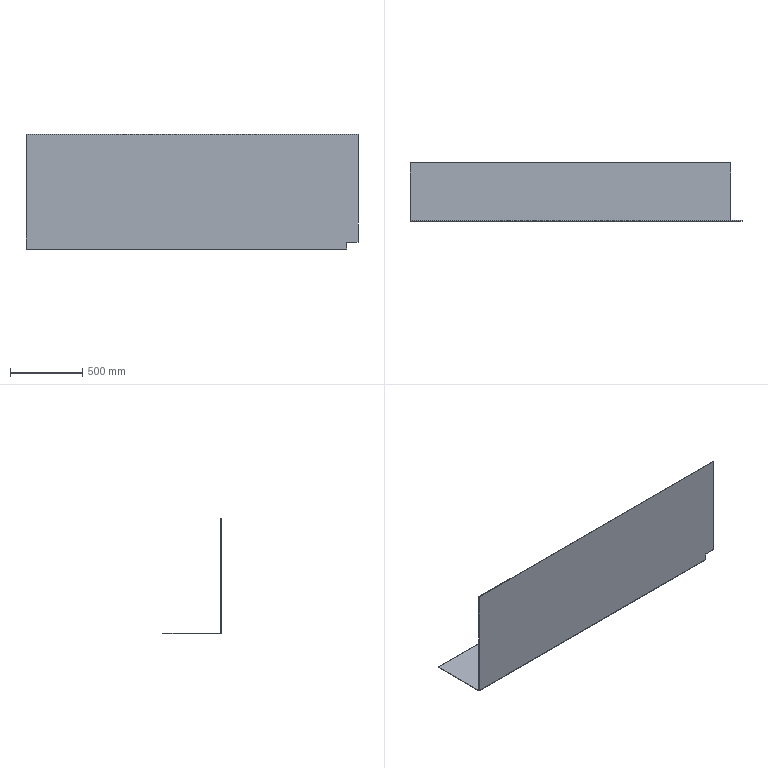Part | STEP file | E3-花纹Plate折弯2 | 1 solid | 14 faces | box 2298 x 403 x 798 mm | volume 8146098 mm3 | plane 12 | cylinder 2 | commonest cylinder face diameters 2 x1 8 x1
STEP:
#1=CARTESIAN_POINT('',(0.,0.,0.));
#2=DIRECTION('',(0.,0.,1.));
#3=DIRECTION('',(1.,0.,0.));
#4=AXIS2_PLACEMENT_3D('',#1,#2,#3);
#5=CARTESIAN_POINT('',(2298.,0.,-746.));
#6=VERTEX_POINT('',#5);
#7=CARTESIAN_POINT('',(2298.,3.,-746.));
#8=VERTEX_POINT('',#7);
#9=CARTESIAN_POINT('',(2298.,3.,-746.));
#10=DIRECTION('',(0.,1.,0.));
#11=VECTOR('',#10,1.);
#12=LINE('',#9,#11);
#13=CARTESIAN_POINT('',(2298.,3.,0.));
#14=DIRECTION('',(1.,0.,0.));
#15=DIRECTION('',(0.,0.,1.));
#16=AXIS2_PLACEMENT_3D('',#13,#14,#15);
#17=PLANE('',#16);
#18=CARTESIAN_POINT('',(-746.,0.));
#19=DIRECTION('',(0.,-1.));
#20=VECTOR('',#19,1.);
#21=LINE('',#18,#20);
#22=(GEOMETRIC_REPRESENTATION_CONTEXT(2)PARAMETRIC_REPRESENTATION_CONTEXT()REPRESENTATION_CONTEXT('',''));
#23=DEFINITIONAL_REPRESENTATION('',(#21),#22);
#24=PCURVE('',#17,#23);
#25=CARTESIAN_POINT('',(2220.,-497.,-746.));
#26=DIRECTION('',(0.,0.,1.));
#27=DIRECTION('',(-1.,0.,0.));
#28=AXIS2_PLACEMENT_3D('',#25,#26,#27);
#29=PLANE('',#28);
#30=CARTESIAN_POINT('',(-78.,-500.));
#31=DIRECTION('',(0.,-1.));
#32=VECTOR('',#31,1.);
#33=LINE('',#30,#32);
#34=(GEOMETRIC_REPRESENTATION_CONTEXT(2)PARAMETRIC_REPRESENTATION_CONTEXT()REPRESENTATION_CONTEXT('',''));
#35=DEFINITIONAL_REPRESENTATION('',(#33),#34);
#36=PCURVE('',#29,#35);
#37=SURFACE_CURVE('',#12,(#24,#36),.PCURVE_S1.);
#38=EDGE_CURVE('',#6,#8,#37,.T.);
#39=ORIENTED_EDGE('',*,*,#38,.T.);
#40=CARTESIAN_POINT('',(2298.,3.,0.));
#41=VERTEX_POINT('',#40);
#42=CARTESIAN_POINT('',(2298.,3.,0.));
#43=DIRECTION('',(0.,0.,1.));
#44=VECTOR('',#43,1.);
#45=LINE('',#42,#44);
#46=CARTESIAN_POINT('',(0.,0.));
#47=DIRECTION('',(1.,0.));
#48=VECTOR('',#47,1.);
#49=LINE('',#46,#48);
#50=(GEOMETRIC_REPRESENTATION_CONTEXT(2)PARAMETRIC_REPRESENTATION_CONTEXT()REPRESENTATION_CONTEXT('',''));
#51=DEFINITIONAL_REPRESENTATION('',(#49),#50);
#52=PCURVE('',#17,#51);
#53=CARTESIAN_POINT('',(0.,3.,0.));
#54=DIRECTION('',(0.,1.,0.));
#55=DIRECTION('',(0.,0.,-1.));
#56=AXIS2_PLACEMENT_3D('',#53,#54,#55);
#57=PLANE('',#56);
#58=CARTESIAN_POINT('',(0.,-2298.));
#59=DIRECTION('',(-1.,0.));
#60=VECTOR('',#59,1.);
#61=LINE('',#58,#60);
#62=(GEOMETRIC_REPRESENTATION_CONTEXT(2)PARAMETRIC_REPRESENTATION_CONTEXT()REPRESENTATION_CONTEXT('',''));
#63=DEFINITIONAL_REPRESENTATION('',(#61),#62);
#64=PCURVE('',#57,#63);
#65=SURFACE_CURVE('',#45,(#52,#64),.PCURVE_S1.);
#66=EDGE_CURVE('',#8,#41,#65,.T.);
#67=ORIENTED_EDGE('',*,*,#66,.T.);
#68=CARTESIAN_POINT('',(2298.,0.,0.));
#69=VERTEX_POINT('',#68);
#70=CARTESIAN_POINT('',(2298.,3.,0.));
#71=DIRECTION('',(0.,1.,0.));
#72=VECTOR('',#71,1.);
#73=LINE('',#70,#72);
#74=CARTESIAN_POINT('',(0.,0.));
#75=DIRECTION('',(0.,-1.));
#76=VECTOR('',#75,1.);
#77=LINE('',#74,#76);
#78=(GEOMETRIC_REPRESENTATION_CONTEXT(2)PARAMETRIC_REPRESENTATION_CONTEXT()REPRESENTATION_CONTEXT('',''));
#79=DEFINITIONAL_REPRESENTATION('',(#77),#78);
#80=PCURVE('',#17,#79);
#81=CARTESIAN_POINT('',(0.,3.,0.));
#82=DIRECTION('',(0.,0.,1.));
#83=DIRECTION('',(-1.,0.,0.));
#84=AXIS2_PLACEMENT_3D('',#81,#82,#83);
#85=PLANE('',#84);
#86=CARTESIAN_POINT('',(-2298.,0.));
#87=DIRECTION('',(0.,-1.));
#88=VECTOR('',#87,1.);
#89=LINE('',#86,#88);
#90=(GEOMETRIC_REPRESENTATION_CONTEXT(2)PARAMETRIC_REPRESENTATION_CONTEXT()REPRESENTATION_CONTEXT('',''));
#91=DEFINITIONAL_REPRESENTATION('',(#89),#90);
#92=PCURVE('',#85,#91);
#93=SURFACE_CURVE('',#73,(#80,#92),.PCURVE_S1.);
#94=EDGE_CURVE('',#69,#41,#93,.T.);
#95=ORIENTED_EDGE('',*,*,#94,.F.);
#96=CARTESIAN_POINT('',(2298.,0.,0.));
#97=DIRECTION('',(0.,0.,1.));
#98=VECTOR('',#97,1.);
#99=LINE('',#96,#98);
#100=CARTESIAN_POINT('',(0.,3.));
#101=DIRECTION('',(1.,0.));
#102=VECTOR('',#101,1.);
#103=LINE('',#100,#102);
#104=(GEOMETRIC_REPRESENTATION_CONTEXT(2)PARAMETRIC_REPRESENTATION_CONTEXT()REPRESENTATION_CONTEXT('',''));
#105=DEFINITIONAL_REPRESENTATION('',(#103),#104);
#106=PCURVE('',#17,#105);
#107=CARTESIAN_POINT('',(0.,0.,0.));
#108=DIRECTION('',(0.,1.,0.));
#109=DIRECTION('',(0.,0.,-1.));
#110=AXIS2_PLACEMENT_3D('',#107,#108,#109);
#111=PLANE('',#110);
#112=CARTESIAN_POINT('',(0.,-2298.));
#113=DIRECTION('',(-1.,0.));
#114=VECTOR('',#113,1.);
#115=LINE('',#112,#114);
#116=(GEOMETRIC_REPRESENTATION_CONTEXT(2)PARAMETRIC_REPRESENTATION_CONTEXT()REPRESENTATION_CONTEXT('',''));
#117=DEFINITIONAL_REPRESENTATION('',(#115),#116);
#118=PCURVE('',#111,#117);
#119=SURFACE_CURVE('',#99,(#106,#118),.PCURVE_S1.);
#120=EDGE_CURVE('',#6,#69,#119,.T.);
#121=ORIENTED_EDGE('',*,*,#120,.F.);
#122=EDGE_LOOP('',(#39,#67,#95,#121));
#123=FACE_BOUND('',#122,.T.);
#124=ADVANCED_FACE('',(#123),#17,.T.);
#125=CARTESIAN_POINT('',(2220.,3.,-746.));
#126=VERTEX_POINT('',#125);
#127=CARTESIAN_POINT('',(2220.,3.,-794.));
#128=VERTEX_POINT('',#127);
#129=CARTESIAN_POINT('',(2220.,3.,0.));
#130=DIRECTION('',(0.,0.,-1.));
#131=VECTOR('',#130,1.);
#132=LINE('',#129,#131);
#133=CARTESIAN_POINT('',(0.,-2220.));
#134=DIRECTION('',(1.,0.));
#135=VECTOR('',#134,1.);
#136=LINE('',#133,#135);
#137=(GEOMETRIC_REPRESENTATION_CONTEXT(2)PARAMETRIC_REPRESENTATION_CONTEXT()REPRESENTATION_CONTEXT('',''));
#138=DEFINITIONAL_REPRESENTATION('',(#136),#137);
#139=PCURVE('',#57,#138);
#140=CARTESIAN_POINT('',(2220.,-497.,-798.));
#141=DIRECTION('',(-1.,0.,0.));
#142=DIRECTION('',(0.,0.,-1.));
#143=AXIS2_PLACEMENT_3D('',#140,#141,#142);
#144=PLANE('',#143);
#145=CARTESIAN_POINT('',(-798.,-500.));
#146=DIRECTION('',(1.,0.));
#147=VECTOR('',#146,1.);
#148=LINE('',#145,#147);
#149=(GEOMETRIC_REPRESENTATION_CONTEXT(2)PARAMETRIC_REPRESENTATION_CONTEXT()REPRESENTATION_CONTEXT('',''));
#150=DEFINITIONAL_REPRESENTATION('',(#148),#149);
#151=PCURVE('',#144,#150);
#152=SURFACE_CURVE('',#132,(#139,#151),.PCURVE_S1.);
#153=EDGE_CURVE('',#126,#128,#152,.T.);
#154=ORIENTED_EDGE('',*,*,#153,.T.);
#155=CARTESIAN_POINT('',(0.,3.,-794.));
#156=VERTEX_POINT('',#155);
#157=CARTESIAN_POINT('',(2298.,3.,-794.));
#158=DIRECTION('',(-1.,0.,0.));
#159=VECTOR('',#158,1.);
#160=LINE('',#157,#159);
#161=CARTESIAN_POINT('',(794.,-2298.));
#162=DIRECTION('',(0.,1.));
#163=VECTOR('',#162,1.);
#164=LINE('',#161,#163);
#165=(GEOMETRIC_REPRESENTATION_CONTEXT(2)PARAMETRIC_REPRESENTATION_CONTEXT()REPRESENTATION_CONTEXT('',''));
#166=DEFINITIONAL_REPRESENTATION('',(#164),#165);
#167=PCURVE('',#57,#166);
#168=CARTESIAN_POINT('',(2298.,4.,-794.));
#169=DIRECTION('',(1.,0.,0.));
#170=DIRECTION('',(0.,0.,-1.));
#171=AXIS2_PLACEMENT_3D('',#168,#169,#170);
#172=CYLINDRICAL_SURFACE('',#171,1.);
#173=CARTESIAN_POINT('',(4.712,0.));
#174=DIRECTION('',(0.,-1.));
#175=VECTOR('',#174,1.);
#176=LINE('',#173,#175);
#177=(GEOMETRIC_REPRESENTATION_CONTEXT(2)PARAMETRIC_REPRESENTATION_CONTEXT()REPRESENTATION_CONTEXT('',''));
#178=DEFINITIONAL_REPRESENTATION('',(#176),#177);
#179=PCURVE('',#172,#178);
#180=SURFACE_CURVE('',#160,(#167,#179),.PCURVE_S1.);
#181=EDGE_CURVE('',#128,#156,#180,.T.);
#182=ORIENTED_EDGE('',*,*,#181,.T.);
#183=CARTESIAN_POINT('',(0.,3.,0.));
#184=VERTEX_POINT('',#183);
#185=CARTESIAN_POINT('',(0.,3.,0.));
#186=DIRECTION('',(0.,0.,-1.));
#187=VECTOR('',#186,1.);
#188=LINE('',#185,#187);
#189=CARTESIAN_POINT('',(0.,0.));
#190=DIRECTION('',(1.,0.));
#191=VECTOR('',#190,1.);
#192=LINE('',#189,#191);
#193=(GEOMETRIC_REPRESENTATION_CONTEXT(2)PARAMETRIC_REPRESENTATION_CONTEXT()REPRESENTATION_CONTEXT('',''));
#194=DEFINITIONAL_REPRESENTATION('',(#192),#193);
#195=PCURVE('',#57,#194);
#196=CARTESIAN_POINT('',(0.,3.,0.));
#197=DIRECTION('',(-1.,0.,0.));
#198=DIRECTION('',(0.,0.,-1.));
#199=AXIS2_PLACEMENT_3D('',#196,#197,#198);
#200=PLANE('',#199);
#201=CARTESIAN_POINT('',(0.,0.));
#202=DIRECTION('',(1.,0.));
#203=VECTOR('',#202,1.);
#204=LINE('',#201,#203);
#205=(GEOMETRIC_REPRESENTATION_CONTEXT(2)PARAMETRIC_REPRESENTATION_CONTEXT()REPRESENTATION_CONTEXT('',''));
#206=DEFINITIONAL_REPRESENTATION('',(#204),#205);
#207=PCURVE('',#200,#206);
#208=SURFACE_CURVE('',#188,(#195,#207),.PCURVE_S1.);
#209=EDGE_CURVE('',#184,#156,#208,.T.);
#210=ORIENTED_EDGE('',*,*,#209,.F.);
#211=CARTESIAN_POINT('',(0.,3.,0.));
#212=DIRECTION('',(-1.,0.,0.));
#213=VECTOR('',#212,1.);
#214=LINE('',#211,#213);
#215=CARTESIAN_POINT('',(0.,0.));
#216=DIRECTION('',(0.,1.));
#217=VECTOR('',#216,1.);
#218=LINE('',#215,#217);
#219=(GEOMETRIC_REPRESENTATION_CONTEXT(2)PARAMETRIC_REPRESENTATION_CONTEXT()REPRESENTATION_CONTEXT('',''));
#220=DEFINITIONAL_REPRESENTATION('',(#218),#219);
#221=PCURVE('',#57,#220);
#222=CARTESIAN_POINT('',(0.,0.));
#223=DIRECTION('',(1.,0.));
#224=VECTOR('',#223,1.);
#225=LINE('',#222,#224);
#226=(GEOMETRIC_REPRESENTATION_CONTEXT(2)PARAMETRIC_REPRESENTATION_CONTEXT()REPRESENTATION_CONTEXT('',''));
#227=DEFINITIONAL_REPRESENTATION('',(#225),#226);
#228=PCURVE('',#85,#227);
#229=SURFACE_CURVE('',#214,(#221,#228),.PCURVE_S1.);
#230=EDGE_CURVE('',#41,#184,#229,.T.);
#231=ORIENTED_EDGE('',*,*,#230,.F.);
#232=ORIENTED_EDGE('',*,*,#66,.F.);
#233=CARTESIAN_POINT('',(0.,3.,-746.));
#234=DIRECTION('',(-1.,0.,0.));
#235=VECTOR('',#234,1.);
#236=LINE('',#233,#235);
#237=CARTESIAN_POINT('',(746.,0.));
#238=DIRECTION('',(0.,1.));
#239=VECTOR('',#238,1.);
#240=LINE('',#237,#239);
#241=(GEOMETRIC_REPRESENTATION_CONTEXT(2)PARAMETRIC_REPRESENTATION_CONTEXT()REPRESENTATION_CONTEXT('',''));
#242=DEFINITIONAL_REPRESENTATION('',(#240),#241);
#243=PCURVE('',#57,#242);
#244=CARTESIAN_POINT('',(2220.,-500.));
#245=DIRECTION('',(1.,0.));
#246=VECTOR('',#245,1.);
#247=LINE('',#244,#246);
#248=(GEOMETRIC_REPRESENTATION_CONTEXT(2)PARAMETRIC_REPRESENTATION_CONTEXT()REPRESENTATION_CONTEXT('',''));
#249=DEFINITIONAL_REPRESENTATION('',(#247),#248);
#250=PCURVE('',#29,#249);
#251=SURFACE_CURVE('',#236,(#243,#250),.PCURVE_S1.);
#252=EDGE_CURVE('',#8,#126,#251,.T.);
#253=ORIENTED_EDGE('',*,*,#252,.T.);
#254=EDGE_LOOP('',(#154,#182,#210,#231,#232,#253));
#255=FACE_BOUND('',#254,.T.);
#256=ADVANCED_FACE('',(#255),#57,.T.);
#257=CARTESIAN_POINT('',(2220.,0.,-746.));
#258=VERTEX_POINT('',#257);
#259=CARTESIAN_POINT('',(0.,0.,-746.));
#260=DIRECTION('',(-1.,0.,0.));
#261=VECTOR('',#260,1.);
#262=LINE('',#259,#261);
#263=CARTESIAN_POINT('',(746.,0.));
#264=DIRECTION('',(0.,1.));
#265=VECTOR('',#264,1.);
#266=LINE('',#263,#265);
#267=(GEOMETRIC_REPRESENTATION_CONTEXT(2)PARAMETRIC_REPRESENTATION_CONTEXT()REPRESENTATION_CONTEXT('',''));
#268=DEFINITIONAL_REPRESENTATION('',(#266),#267);
#269=PCURVE('',#111,#268);
#270=CARTESIAN_POINT('',(2220.,-497.));
#271=DIRECTION('',(1.,0.));
#272=VECTOR('',#271,1.);
#273=LINE('',#270,#272);
#274=(GEOMETRIC_REPRESENTATION_CONTEXT(2)PARAMETRIC_REPRESENTATION_CONTEXT()REPRESENTATION_CONTEXT('',''));
#275=DEFINITIONAL_REPRESENTATION('',(#273),#274);
#276=PCURVE('',#29,#275);
#277=SURFACE_CURVE('',#262,(#269,#276),.PCURVE_S1.);
#278=EDGE_CURVE('',#6,#258,#277,.T.);
#279=ORIENTED_EDGE('',*,*,#278,.F.);
#280=ORIENTED_EDGE('',*,*,#120,.T.);
#281=CARTESIAN_POINT('',(0.,0.,0.));
#282=VERTEX_POINT('',#281);
#283=CARTESIAN_POINT('',(0.,0.,0.));
#284=DIRECTION('',(-1.,0.,0.));
#285=VECTOR('',#284,1.);
#286=LINE('',#283,#285);
#287=CARTESIAN_POINT('',(0.,0.));
#288=DIRECTION('',(0.,1.));
#289=VECTOR('',#288,1.);
#290=LINE('',#287,#289);
#291=(GEOMETRIC_REPRESENTATION_CONTEXT(2)PARAMETRIC_REPRESENTATION_CONTEXT()REPRESENTATION_CONTEXT('',''));
#292=DEFINITIONAL_REPRESENTATION('',(#290),#291);
#293=PCURVE('',#111,#292);
#294=CARTESIAN_POINT('',(0.,3.));
#295=DIRECTION('',(1.,0.));
#296=VECTOR('',#295,1.);
#297=LINE('',#294,#296);
#298=(GEOMETRIC_REPRESENTATION_CONTEXT(2)PARAMETRIC_REPRESENTATION_CONTEXT()REPRESENTATION_CONTEXT('',''));
#299=DEFINITIONAL_REPRESENTATION('',(#297),#298);
#300=PCURVE('',#85,#299);
#301=SURFACE_CURVE('',#286,(#293,#300),.PCURVE_S1.);
#302=EDGE_CURVE('',#69,#282,#301,.T.);
#303=ORIENTED_EDGE('',*,*,#302,.T.);
#304=CARTESIAN_POINT('',(0.,0.,-794.));
#305=VERTEX_POINT('',#304);
#306=CARTESIAN_POINT('',(0.,0.,0.));
#307=DIRECTION('',(0.,0.,-1.));
#308=VECTOR('',#307,1.);
#309=LINE('',#306,#308);
#310=CARTESIAN_POINT('',(0.,0.));
#311=DIRECTION('',(1.,0.));
#312=VECTOR('',#311,1.);
#313=LINE('',#310,#312);
#314=(GEOMETRIC_REPRESENTATION_CONTEXT(2)PARAMETRIC_REPRESENTATION_CONTEXT()REPRESENTATION_CONTEXT('',''));
#315=DEFINITIONAL_REPRESENTATION('',(#313),#314);
#316=PCURVE('',#111,#315);
#317=CARTESIAN_POINT('',(0.,3.));
#318=DIRECTION('',(1.,0.));
#319=VECTOR('',#318,1.);
#320=LINE('',#317,#319);
#321=(GEOMETRIC_REPRESENTATION_CONTEXT(2)PARAMETRIC_REPRESENTATION_CONTEXT()REPRESENTATION_CONTEXT('',''));
#322=DEFINITIONAL_REPRESENTATION('',(#320),#321);
#323=PCURVE('',#200,#322);
#324=SURFACE_CURVE('',#309,(#316,#323),.PCURVE_S1.);
#325=EDGE_CURVE('',#282,#305,#324,.T.);
#326=ORIENTED_EDGE('',*,*,#325,.T.);
#327=CARTESIAN_POINT('',(2220.,0.,-794.));
#328=VERTEX_POINT('',#327);
#329=CARTESIAN_POINT('',(2298.,0.,-794.));
#330=DIRECTION('',(-1.,0.,0.));
#331=VECTOR('',#330,1.);
#332=LINE('',#329,#331);
#333=CARTESIAN_POINT('',(794.,-2298.));
#334=DIRECTION('',(0.,1.));
#335=VECTOR('',#334,1.);
#336=LINE('',#333,#335);
#337=(GEOMETRIC_REPRESENTATION_CONTEXT(2)PARAMETRIC_REPRESENTATION_CONTEXT()REPRESENTATION_CONTEXT('',''));
#338=DEFINITIONAL_REPRESENTATION('',(#336),#337);
#339=PCURVE('',#111,#338);
#340=CARTESIAN_POINT('',(2298.,4.,-794.));
#341=DIRECTION('',(1.,0.,0.));
#342=DIRECTION('',(0.,0.,-1.));
#343=AXIS2_PLACEMENT_3D('',#340,#341,#342);
#344=CYLINDRICAL_SURFACE('',#343,4.);
#345=CARTESIAN_POINT('',(4.712,0.));
#346=DIRECTION('',(0.,-1.));
#347=VECTOR('',#346,1.);
#348=LINE('',#345,#347);
#349=(GEOMETRIC_REPRESENTATION_CONTEXT(2)PARAMETRIC_REPRESENTATION_CONTEXT()REPRESENTATION_CONTEXT('',''));
#350=DEFINITIONAL_REPRESENTATION('',(#348),#349);
#351=PCURVE('',#344,#350);
#352=SURFACE_CURVE('',#332,(#339,#351),.PCURVE_S1.);
#353=EDGE_CURVE('',#328,#305,#352,.T.);
#354=ORIENTED_EDGE('',*,*,#353,.F.);
#355=CARTESIAN_POINT('',(2220.,0.,0.));
#356=DIRECTION('',(0.,0.,-1.));
#357=VECTOR('',#356,1.);
#358=LINE('',#355,#357);
#359=CARTESIAN_POINT('',(0.,-2220.));
#360=DIRECTION('',(1.,0.));
#361=VECTOR('',#360,1.);
#362=LINE('',#359,#361);
#363=(GEOMETRIC_REPRESENTATION_CONTEXT(2)PARAMETRIC_REPRESENTATION_CONTEXT()REPRESENTATION_CONTEXT('',''));
#364=DEFINITIONAL_REPRESENTATION('',(#362),#363);
#365=PCURVE('',#111,#364);
#366=CARTESIAN_POINT('',(-798.,-497.));
#367=DIRECTION('',(1.,0.));
#368=VECTOR('',#367,1.);
#369=LINE('',#366,#368);
#370=(GEOMETRIC_REPRESENTATION_CONTEXT(2)PARAMETRIC_REPRESENTATION_CONTEXT()REPRESENTATION_CONTEXT('',''));
#371=DEFINITIONAL_REPRESENTATION('',(#369),#370);
#372=PCURVE('',#144,#371);
#373=SURFACE_CURVE('',#358,(#365,#372),.PCURVE_S1.);
#374=EDGE_CURVE('',#258,#328,#373,.T.);
#375=ORIENTED_EDGE('',*,*,#374,.F.);
#376=EDGE_LOOP('',(#279,#280,#303,#326,#354,#375));
#377=FACE_BOUND('',#376,.T.);
#378=ADVANCED_FACE('',(#377),#111,.F.);
#379=ORIENTED_EDGE('',*,*,#94,.T.);
#380=ORIENTED_EDGE('',*,*,#230,.T.);
#381=CARTESIAN_POINT('',(0.,3.,0.));
#382=DIRECTION('',(0.,1.,0.));
#383=VECTOR('',#382,1.);
#384=LINE('',#381,#383);
#385=CARTESIAN_POINT('',(0.,0.));
#386=DIRECTION('',(0.,-1.));
#387=VECTOR('',#386,1.);
#388=LINE('',#385,#387);
#389=(GEOMETRIC_REPRESENTATION_CONTEXT(2)PARAMETRIC_REPRESENTATION_CONTEXT()REPRESENTATION_CONTEXT('',''));
#390=DEFINITIONAL_REPRESENTATION('',(#388),#389);
#391=PCURVE('',#85,#390);
#392=CARTESIAN_POINT('',(0.,0.));
#393=DIRECTION('',(0.,-1.));
#394=VECTOR('',#393,1.);
#395=LINE('',#392,#394);
#396=(GEOMETRIC_REPRESENTATION_CONTEXT(2)PARAMETRIC_REPRESENTATION_CONTEXT()REPRESENTATION_CONTEXT('',''));
#397=DEFINITIONAL_REPRESENTATION('',(#395),#396);
#398=PCURVE('',#200,#397);
#399=SURFACE_CURVE('',#384,(#391,#398),.PCURVE_S1.);
#400=EDGE_CURVE('',#282,#184,#399,.T.);
#401=ORIENTED_EDGE('',*,*,#400,.F.);
#402=ORIENTED_EDGE('',*,*,#302,.F.);
#403=EDGE_LOOP('',(#379,#380,#401,#402));
#404=FACE_BOUND('',#403,.T.);
#405=ADVANCED_FACE('',(#404),#85,.T.);
#406=CARTESIAN_POINT('',(0.,3.,-794.));
#407=DIRECTION('',(0.,-1.,0.));
#408=VECTOR('',#407,1.);
#409=LINE('',#406,#408);
#410=CARTESIAN_POINT('',(794.,0.));
#411=DIRECTION('',(0.,1.));
#412=VECTOR('',#411,1.);
#413=LINE('',#410,#412);
#414=(GEOMETRIC_REPRESENTATION_CONTEXT(2)PARAMETRIC_REPRESENTATION_CONTEXT()REPRESENTATION_CONTEXT('',''));
#415=DEFINITIONAL_REPRESENTATION('',(#413),#414);
#416=PCURVE('',#200,#415);
#417=CARTESIAN_POINT('',(0.,4.,-794.));
#418=DIRECTION('',(-1.,0.,0.));
#419=DIRECTION('',(0.,0.,-1.));
#420=AXIS2_PLACEMENT_3D('',#417,#418,#419);
#421=PLANE('',#420);
#422=CARTESIAN_POINT('',(0.,1.));
#423=DIRECTION('',(0.,1.));
#424=VECTOR('',#423,1.);
#425=LINE('',#422,#424);
#426=(GEOMETRIC_REPRESENTATION_CONTEXT(2)PARAMETRIC_REPRESENTATION_CONTEXT()REPRESENTATION_CONTEXT('',''));
#427=DEFINITIONAL_REPRESENTATION('',(#425),#426);
#428=PCURVE('',#421,#427);
#429=SURFACE_CURVE('',#409,(#416,#428),.PCURVE_S1.);
#430=EDGE_CURVE('',#156,#305,#429,.T.);
#431=ORIENTED_EDGE('',*,*,#430,.T.);
#432=ORIENTED_EDGE('',*,*,#325,.F.);
#433=ORIENTED_EDGE('',*,*,#400,.T.);
#434=ORIENTED_EDGE('',*,*,#209,.T.);
#435=EDGE_LOOP('',(#431,#432,#433,#434));
#436=FACE_BOUND('',#435,.T.);
#437=ADVANCED_FACE('',(#436),#200,.T.);
#438=CARTESIAN_POINT('',(0.,4.,-795.));
#439=VERTEX_POINT('',#438);
#440=CARTESIAN_POINT('',(0.,4.,-798.));
#441=VERTEX_POINT('',#440);
#442=CARTESIAN_POINT('',(0.,4.,-798.));
#443=DIRECTION('',(0.,0.,-1.));
#444=VECTOR('',#443,1.);
#445=LINE('',#442,#444);
#446=CARTESIAN_POINT('',(4.,0.));
#447=DIRECTION('',(1.,0.));
#448=VECTOR('',#447,1.);
#449=LINE('',#446,#448);
#450=(GEOMETRIC_REPRESENTATION_CONTEXT(2)PARAMETRIC_REPRESENTATION_CONTEXT()REPRESENTATION_CONTEXT('',''));
#451=DEFINITIONAL_REPRESENTATION('',(#449),#450);
#452=PCURVE('',#421,#451);
#453=CARTESIAN_POINT('',(0.,3.,-798.));
#454=DIRECTION('',(1.,0.,0.));
#455=DIRECTION('',(0.,0.,1.));
#456=AXIS2_PLACEMENT_3D('',#453,#454,#455);
#457=PLANE('',#456);
#458=CARTESIAN_POINT('',(0.,-1.));
#459=DIRECTION('',(-1.,0.));
#460=VECTOR('',#459,1.);
#461=LINE('',#458,#460);
#462=(GEOMETRIC_REPRESENTATION_CONTEXT(2)PARAMETRIC_REPRESENTATION_CONTEXT()REPRESENTATION_CONTEXT('',''));
#463=DEFINITIONAL_REPRESENTATION('',(#461),#462);
#464=PCURVE('',#457,#463);
#465=SURFACE_CURVE('',#445,(#452,#464),.PCURVE_S1.);
#466=EDGE_CURVE('',#439,#441,#465,.T.);
#467=ORIENTED_EDGE('',*,*,#466,.T.);
#468=CARTESIAN_POINT('',(0.,4.,-794.));
#469=DIRECTION('',(1.,0.,0.));
#470=DIRECTION('',(0.,0.,1.));
#471=AXIS2_PLACEMENT_3D('',#468,#469,#470);
#472=CIRCLE('',#471,4.);
#473=CARTESIAN_POINT('',(-4.,0.));
#474=CARTESIAN_POINT('',(-4.,6.928));
#475=CARTESIAN_POINT('',(2.,3.464));
#476=CARTESIAN_POINT('',(8.,0.));
#477=CARTESIAN_POINT('',(2.,-3.464));
#478=CARTESIAN_POINT('',(-4.,-6.928));
#479=CARTESIAN_POINT('',(-4.,0.));
#480=(BOUNDED_CURVE()B_SPLINE_CURVE(2,(#473,#474,#475,#476,#477,#478,#479),.UNSPECIFIED.,.T.,.F.)B_SPLINE_CURVE_WITH_KNOTS((1,2,2,2,2,1),(-2.094,0.,2.094,4.189,6.283,8.378),.UNSPECIFIED.)CURVE()GEOMETRIC_REPRESENTATION_ITEM()RATIONAL_B_SPLINE_CURVE((1.,0.5,1.,0.5,1.,0.5,1.))REPRESENTATION_ITEM(''));
#481=(GEOMETRIC_REPRESENTATION_CONTEXT(2)PARAMETRIC_REPRESENTATION_CONTEXT()REPRESENTATION_CONTEXT('',''));
#482=DEFINITIONAL_REPRESENTATION('',(#480),#481);
#483=PCURVE('',#421,#482);
#484=CARTESIAN_POINT('',(3.142,-2298.));
#485=DIRECTION('',(1.,0.));
#486=VECTOR('',#485,1.);
#487=LINE('',#484,#486);
#488=(GEOMETRIC_REPRESENTATION_CONTEXT(2)PARAMETRIC_REPRESENTATION_CONTEXT()REPRESENTATION_CONTEXT('',''));
#489=DEFINITIONAL_REPRESENTATION('',(#487),#488);
#490=PCURVE('',#344,#489);
#491=SURFACE_CURVE('',#472,(#483,#490),.PCURVE_S1.);
#492=EDGE_CURVE('',#305,#441,#491,.T.);
#493=ORIENTED_EDGE('',*,*,#492,.F.);
#494=ORIENTED_EDGE('',*,*,#430,.F.);
#495=CARTESIAN_POINT('',(0.,4.,-794.));
#496=DIRECTION('',(1.,0.,0.));
#497=DIRECTION('',(0.,0.,1.));
#498=AXIS2_PLACEMENT_3D('',#495,#496,#497);
#499=CIRCLE('',#498,1.);
#500=CARTESIAN_POINT('',(-1.,0.));
#501=CARTESIAN_POINT('',(-1.,1.732));
#502=CARTESIAN_POINT('',(0.5,0.866));
#503=CARTESIAN_POINT('',(2.,0.));
#504=CARTESIAN_POINT('',(0.5,-0.866));
#505=CARTESIAN_POINT('',(-1.,-1.732));
#506=CARTESIAN_POINT('',(-1.,0.));
#507=(BOUNDED_CURVE()B_SPLINE_CURVE(2,(#500,#501,#502,#503,#504,#505,#506),.UNSPECIFIED.,.T.,.F.)B_SPLINE_CURVE_WITH_KNOTS((1,2,2,2,2,1),(-2.094,0.,2.094,4.189,6.283,8.378),.UNSPECIFIED.)CURVE()GEOMETRIC_REPRESENTATION_ITEM()RATIONAL_B_SPLINE_CURVE((1.,0.5,1.,0.5,1.,0.5,1.))REPRESENTATION_ITEM(''));
#508=(GEOMETRIC_REPRESENTATION_CONTEXT(2)PARAMETRIC_REPRESENTATION_CONTEXT()REPRESENTATION_CONTEXT('',''));
#509=DEFINITIONAL_REPRESENTATION('',(#507),#508);
#510=PCURVE('',#421,#509);
#511=CARTESIAN_POINT('',(3.142,-2298.));
#512=DIRECTION('',(1.,0.));
#513=VECTOR('',#512,1.);
#514=LINE('',#511,#513);
#515=(GEOMETRIC_REPRESENTATION_CONTEXT(2)PARAMETRIC_REPRESENTATION_CONTEXT()REPRESENTATION_CONTEXT('',''));
#516=DEFINITIONAL_REPRESENTATION('',(#514),#515);
#517=PCURVE('',#172,#516);
#518=SURFACE_CURVE('',#499,(#510,#517),.PCURVE_S1.);
#519=EDGE_CURVE('',#156,#439,#518,.T.);
#520=ORIENTED_EDGE('',*,*,#519,.T.);
#521=EDGE_LOOP('',(#467,#493,#494,#520));
#522=FACE_BOUND('',#521,.T.);
#523=ADVANCED_FACE('',(#522),#421,.T.);
#524=CARTESIAN_POINT('',(2220.,4.,-798.));
#525=VERTEX_POINT('',#524);
#526=CARTESIAN_POINT('',(2220.,4.,-794.));
#527=DIRECTION('',(-1.,0.,0.));
#528=DIRECTION('',(0.,0.,-1.));
#529=AXIS2_PLACEMENT_3D('',#526,#527,#528);
#530=CIRCLE('',#529,4.);
#531=CARTESIAN_POINT('',(6.283,-78.));
#532=DIRECTION('',(-1.,0.));
#533=VECTOR('',#532,1.);
#534=LINE('',#531,#533);
#535=(GEOMETRIC_REPRESENTATION_CONTEXT(2)PARAMETRIC_REPRESENTATION_CONTEXT()REPRESENTATION_CONTEXT('',''));
#536=DEFINITIONAL_REPRESENTATION('',(#534),#535);
#537=PCURVE('',#344,#536);
#538=CARTESIAN_POINT('',(-4.,-501.));
#539=DIRECTION('',(1.,0.));
#540=AXIS2_PLACEMENT_2D('',#538,#539);
#541=CIRCLE('',#540,4.);
#542=(GEOMETRIC_REPRESENTATION_CONTEXT(2)PARAMETRIC_REPRESENTATION_CONTEXT()REPRESENTATION_CONTEXT('',''));
#543=DEFINITIONAL_REPRESENTATION('',(#541),#542);
#544=PCURVE('',#144,#543);
#545=SURFACE_CURVE('',#530,(#537,#544),.PCURVE_S1.);
#546=EDGE_CURVE('',#525,#328,#545,.T.);
#547=ORIENTED_EDGE('',*,*,#546,.T.);
#548=ORIENTED_EDGE('',*,*,#353,.T.);
#549=ORIENTED_EDGE('',*,*,#492,.T.);
#550=CARTESIAN_POINT('',(0.,4.,-798.));
#551=DIRECTION('',(-1.,0.,0.));
#552=VECTOR('',#551,1.);
#553=LINE('',#550,#552);
#554=CARTESIAN_POINT('',(6.283,-2298.));
#555=DIRECTION('',(0.,-1.));
#556=VECTOR('',#555,1.);
#557=LINE('',#554,#556);
#558=(GEOMETRIC_REPRESENTATION_CONTEXT(2)PARAMETRIC_REPRESENTATION_CONTEXT()REPRESENTATION_CONTEXT('',''));
#559=DEFINITIONAL_REPRESENTATION('',(#557),#558);
#560=PCURVE('',#344,#559);
#561=CARTESIAN_POINT('',(0.,0.,-798.));
#562=DIRECTION('',(0.,0.,1.));
#563=DIRECTION('',(-1.,0.,0.));
#564=AXIS2_PLACEMENT_3D('',#561,#562,#563);
#565=PLANE('',#564);
#566=CARTESIAN_POINT('',(0.,-4.));
#567=DIRECTION('',(1.,0.));
#568=VECTOR('',#567,1.);
#569=LINE('',#566,#568);
#570=(GEOMETRIC_REPRESENTATION_CONTEXT(2)PARAMETRIC_REPRESENTATION_CONTEXT()REPRESENTATION_CONTEXT('',''));
#571=DEFINITIONAL_REPRESENTATION('',(#569),#570);
#572=PCURVE('',#565,#571);
#573=SURFACE_CURVE('',#553,(#560,#572),.PCURVE_S1.);
#574=EDGE_CURVE('',#525,#441,#573,.T.);
#575=ORIENTED_EDGE('',*,*,#574,.F.);
#576=EDGE_LOOP('',(#547,#548,#549,#575));
#577=FACE_BOUND('',#576,.T.);
#578=ADVANCED_FACE('',(#577),#344,.T.);
#579=CARTESIAN_POINT('',(2220.,4.,-795.));
#580=VERTEX_POINT('',#579);
#581=CARTESIAN_POINT('',(2220.,4.,-794.));
#582=DIRECTION('',(-1.,0.,0.));
#583=DIRECTION('',(0.,0.,-1.));
#584=AXIS2_PLACEMENT_3D('',#581,#582,#583);
#585=CIRCLE('',#584,1.);
#586=CARTESIAN_POINT('',(6.283,-78.));
#587=DIRECTION('',(-1.,0.));
#588=VECTOR('',#587,1.);
#589=LINE('',#586,#588);
#590=(GEOMETRIC_REPRESENTATION_CONTEXT(2)PARAMETRIC_REPRESENTATION_CONTEXT()REPRESENTATION_CONTEXT('',''));
#591=DEFINITIONAL_REPRESENTATION('',(#589),#590);
#592=PCURVE('',#172,#591);
#593=CARTESIAN_POINT('',(-4.,-501.));
#594=DIRECTION('',(1.,0.));
#595=AXIS2_PLACEMENT_2D('',#593,#594);
#596=CIRCLE('',#595,1.);
#597=(GEOMETRIC_REPRESENTATION_CONTEXT(2)PARAMETRIC_REPRESENTATION_CONTEXT()REPRESENTATION_CONTEXT('',''));
#598=DEFINITIONAL_REPRESENTATION('',(#596),#597);
#599=PCURVE('',#144,#598);
#600=SURFACE_CURVE('',#585,(#592,#599),.PCURVE_S1.);
#601=EDGE_CURVE('',#580,#128,#600,.T.);
#602=ORIENTED_EDGE('',*,*,#601,.T.);
#603=ORIENTED_EDGE('',*,*,#181,.T.);
#604=ORIENTED_EDGE('',*,*,#519,.T.);
#605=CARTESIAN_POINT('',(0.,4.,-795.));
#606=DIRECTION('',(1.,0.,0.));
#607=VECTOR('',#606,1.);
#608=LINE('',#605,#607);
#609=CARTESIAN_POINT('',(6.283,-2298.));
#610=DIRECTION('',(0.,1.));
#611=VECTOR('',#610,1.);
#612=LINE('',#609,#611);
#613=(GEOMETRIC_REPRESENTATION_CONTEXT(2)PARAMETRIC_REPRESENTATION_CONTEXT()REPRESENTATION_CONTEXT('',''));
#614=DEFINITIONAL_REPRESENTATION('',(#612),#613);
#615=PCURVE('',#172,#614);
#616=CARTESIAN_POINT('',(0.,0.,-795.));
#617=DIRECTION('',(0.,0.,1.));
#618=DIRECTION('',(-1.,0.,0.));
#619=AXIS2_PLACEMENT_3D('',#616,#617,#618);
#620=PLANE('',#619);
#621=CARTESIAN_POINT('',(0.,-4.));
#622=DIRECTION('',(-1.,0.));
#623=VECTOR('',#622,1.);
#624=LINE('',#621,#623);
#625=(GEOMETRIC_REPRESENTATION_CONTEXT(2)PARAMETRIC_REPRESENTATION_CONTEXT()REPRESENTATION_CONTEXT('',''));
#626=DEFINITIONAL_REPRESENTATION('',(#624),#625);
#627=PCURVE('',#620,#626);
#628=SURFACE_CURVE('',#608,(#615,#627),.PCURVE_S1.);
#629=EDGE_CURVE('',#439,#580,#628,.T.);
#630=ORIENTED_EDGE('',*,*,#629,.T.);
#631=EDGE_LOOP('',(#602,#603,#604,#630));
#632=FACE_BOUND('',#631,.F.);
#633=ADVANCED_FACE('',(#632),#172,.F.);
#634=ORIENTED_EDGE('',*,*,#466,.F.);
#635=CARTESIAN_POINT('',(0.,403.,-795.));
#636=VERTEX_POINT('',#635);
#637=CARTESIAN_POINT('',(0.,3.,-795.));
#638=DIRECTION('',(0.,-1.,0.));
#639=VECTOR('',#638,1.);
#640=LINE('',#637,#639);
#641=CARTESIAN_POINT('',(3.,0.));
#642=DIRECTION('',(0.,1.));
#643=VECTOR('',#642,1.);
#644=LINE('',#641,#643);
#645=(GEOMETRIC_REPRESENTATION_CONTEXT(2)PARAMETRIC_REPRESENTATION_CONTEXT()REPRESENTATION_CONTEXT('',''));
#646=DEFINITIONAL_REPRESENTATION('',(#644),#645);
#647=PCURVE('',#457,#646);
#648=CARTESIAN_POINT('',(0.,-3.));
#649=DIRECTION('',(0.,1.));
#650=VECTOR('',#649,1.);
#651=LINE('',#648,#650);
#652=(GEOMETRIC_REPRESENTATION_CONTEXT(2)PARAMETRIC_REPRESENTATION_CONTEXT()REPRESENTATION_CONTEXT('',''));
#653=DEFINITIONAL_REPRESENTATION('',(#651),#652);
#654=PCURVE('',#620,#653);
#655=SURFACE_CURVE('',#640,(#647,#654),.PCURVE_S1.);
#656=EDGE_CURVE('',#636,#439,#655,.T.);
#657=ORIENTED_EDGE('',*,*,#656,.F.);
#658=CARTESIAN_POINT('',(0.,403.,-798.));
#659=VERTEX_POINT('',#658);
#660=CARTESIAN_POINT('',(0.,403.,-798.));
#661=DIRECTION('',(0.,0.,1.));
#662=VECTOR('',#661,1.);
#663=LINE('',#660,#662);
#664=CARTESIAN_POINT('',(0.,-400.));
#665=DIRECTION('',(1.,0.));
#666=VECTOR('',#665,1.);
#667=LINE('',#664,#666);
#668=(GEOMETRIC_REPRESENTATION_CONTEXT(2)PARAMETRIC_REPRESENTATION_CONTEXT()REPRESENTATION_CONTEXT('',''));
#669=DEFINITIONAL_REPRESENTATION('',(#667),#668);
#670=PCURVE('',#457,#669);
#671=CARTESIAN_POINT('',(0.,403.,-798.));
#672=DIRECTION('',(0.,-1.,0.));
#673=DIRECTION('',(0.,0.,1.));
#674=AXIS2_PLACEMENT_3D('',#671,#672,#673);
#675=PLANE('',#674);
#676=CARTESIAN_POINT('',(0.,0.));
#677=DIRECTION('',(1.,0.));
#678=VECTOR('',#677,1.);
#679=LINE('',#676,#678);
#680=(GEOMETRIC_REPRESENTATION_CONTEXT(2)PARAMETRIC_REPRESENTATION_CONTEXT()REPRESENTATION_CONTEXT('',''));
#681=DEFINITIONAL_REPRESENTATION('',(#679),#680);
#682=PCURVE('',#675,#681);
#683=SURFACE_CURVE('',#663,(#670,#682),.PCURVE_S1.);
#684=EDGE_CURVE('',#659,#636,#683,.T.);
#685=ORIENTED_EDGE('',*,*,#684,.F.);
#686=CARTESIAN_POINT('',(0.,0.,-798.));
#687=DIRECTION('',(0.,-1.,0.));
#688=VECTOR('',#687,1.);
#689=LINE('',#686,#688);
#690=CARTESIAN_POINT('',(0.,3.));
#691=DIRECTION('',(0.,1.));
#692=VECTOR('',#691,1.);
#693=LINE('',#690,#692);
#694=(GEOMETRIC_REPRESENTATION_CONTEXT(2)PARAMETRIC_REPRESENTATION_CONTEXT()REPRESENTATION_CONTEXT('',''));
#695=DEFINITIONAL_REPRESENTATION('',(#693),#694);
#696=PCURVE('',#457,#695);
#697=CARTESIAN_POINT('',(0.,0.));
#698=DIRECTION('',(0.,1.));
#699=VECTOR('',#698,1.);
#700=LINE('',#697,#699);
#701=(GEOMETRIC_REPRESENTATION_CONTEXT(2)PARAMETRIC_REPRESENTATION_CONTEXT()REPRESENTATION_CONTEXT('',''));
#702=DEFINITIONAL_REPRESENTATION('',(#700),#701);
#703=PCURVE('',#565,#702);
#704=SURFACE_CURVE('',#689,(#696,#703),.PCURVE_S1.);
#705=EDGE_CURVE('',#659,#441,#704,.T.);
#706=ORIENTED_EDGE('',*,*,#705,.T.);
#707=EDGE_LOOP('',(#634,#657,#685,#706));
#708=FACE_BOUND('',#707,.T.);
#709=ADVANCED_FACE('',(#708),#457,.F.);
#710=ORIENTED_EDGE('',*,*,#574,.T.);
#711=ORIENTED_EDGE('',*,*,#705,.F.);
#712=CARTESIAN_POINT('',(2220.,403.,-798.));
#713=VERTEX_POINT('',#712);
#714=CARTESIAN_POINT('',(0.,403.,-798.));
#715=DIRECTION('',(-1.,0.,0.));
#716=VECTOR('',#715,1.);
#717=LINE('',#714,#716);
#718=CARTESIAN_POINT('',(0.,-403.));
#719=DIRECTION('',(1.,0.));
#720=VECTOR('',#719,1.);
#721=LINE('',#718,#720);
#722=(GEOMETRIC_REPRESENTATION_CONTEXT(2)PARAMETRIC_REPRESENTATION_CONTEXT()REPRESENTATION_CONTEXT('',''));
#723=DEFINITIONAL_REPRESENTATION('',(#721),#722);
#724=PCURVE('',#565,#723);
#725=CARTESIAN_POINT('',(0.,0.));
#726=DIRECTION('',(0.,1.));
#727=VECTOR('',#726,1.);
#728=LINE('',#725,#727);
#729=(GEOMETRIC_REPRESENTATION_CONTEXT(2)PARAMETRIC_REPRESENTATION_CONTEXT()REPRESENTATION_CONTEXT('',''));
#730=DEFINITIONAL_REPRESENTATION('',(#728),#729);
#731=PCURVE('',#675,#730);
#732=SURFACE_CURVE('',#717,(#724,#731),.PCURVE_S1.);
#733=EDGE_CURVE('',#713,#659,#732,.T.);
#734=ORIENTED_EDGE('',*,*,#733,.F.);
#735=CARTESIAN_POINT('',(2220.,-497.,-798.));
#736=DIRECTION('',(0.,1.,0.));
#737=VECTOR('',#736,1.);
#738=LINE('',#735,#737);
#739=CARTESIAN_POINT('',(-2220.,497.));
#740=DIRECTION('',(0.,-1.));
#741=VECTOR('',#740,1.);
#742=LINE('',#739,#741);
#743=(GEOMETRIC_REPRESENTATION_CONTEXT(2)PARAMETRIC_REPRESENTATION_CONTEXT()REPRESENTATION_CONTEXT('',''));
#744=DEFINITIONAL_REPRESENTATION('',(#742),#743);
#745=PCURVE('',#565,#744);
#746=CARTESIAN_POINT('',(0.,0.));
#747=DIRECTION('',(0.,-1.));
#748=VECTOR('',#747,1.);
#749=LINE('',#746,#748);
#750=(GEOMETRIC_REPRESENTATION_CONTEXT(2)PARAMETRIC_REPRESENTATION_CONTEXT()REPRESENTATION_CONTEXT('',''));
#751=DEFINITIONAL_REPRESENTATION('',(#749),#750);
#752=PCURVE('',#144,#751);
#753=SURFACE_CURVE('',#738,(#745,#752),.PCURVE_S1.);
#754=EDGE_CURVE('',#525,#713,#753,.T.);
#755=ORIENTED_EDGE('',*,*,#754,.F.);
#756=EDGE_LOOP('',(#710,#711,#734,#755));
#757=FACE_BOUND('',#756,.T.);
#758=ADVANCED_FACE('',(#757),#565,.F.);
#759=CARTESIAN_POINT('',(2220.,403.,-795.));
#760=VERTEX_POINT('',#759);
#761=CARTESIAN_POINT('',(2220.,0.,-795.));
#762=DIRECTION('',(0.,1.,0.));
#763=VECTOR('',#762,1.);
#764=LINE('',#761,#763);
#765=CARTESIAN_POINT('',(-2220.,0.));
#766=DIRECTION('',(0.,-1.));
#767=VECTOR('',#766,1.);
#768=LINE('',#765,#767);
#769=(GEOMETRIC_REPRESENTATION_CONTEXT(2)PARAMETRIC_REPRESENTATION_CONTEXT()REPRESENTATION_CONTEXT('',''));
#770=DEFINITIONAL_REPRESENTATION('',(#768),#769);
#771=PCURVE('',#620,#770);
#772=CARTESIAN_POINT('',(-3.,-497.));
#773=DIRECTION('',(0.,-1.));
#774=VECTOR('',#773,1.);
#775=LINE('',#772,#774);
#776=(GEOMETRIC_REPRESENTATION_CONTEXT(2)PARAMETRIC_REPRESENTATION_CONTEXT()REPRESENTATION_CONTEXT('',''));
#777=DEFINITIONAL_REPRESENTATION('',(#775),#776);
#778=PCURVE('',#144,#777);
#779=SURFACE_CURVE('',#764,(#771,#778),.PCURVE_S1.);
#780=EDGE_CURVE('',#580,#760,#779,.T.);
#781=ORIENTED_EDGE('',*,*,#780,.T.);
#782=CARTESIAN_POINT('',(0.,403.,-795.));
#783=DIRECTION('',(-1.,0.,0.));
#784=VECTOR('',#783,1.);
#785=LINE('',#782,#784);
#786=CARTESIAN_POINT('',(0.,-403.));
#787=DIRECTION('',(1.,0.));
#788=VECTOR('',#787,1.);
#789=LINE('',#786,#788);
#790=(GEOMETRIC_REPRESENTATION_CONTEXT(2)PARAMETRIC_REPRESENTATION_CONTEXT()REPRESENTATION_CONTEXT('',''));
#791=DEFINITIONAL_REPRESENTATION('',(#789),#790);
#792=PCURVE('',#620,#791);
#793=CARTESIAN_POINT('',(3.,0.));
#794=DIRECTION('',(0.,1.));
#795=VECTOR('',#794,1.);
#796=LINE('',#793,#795);
#797=(GEOMETRIC_REPRESENTATION_CONTEXT(2)PARAMETRIC_REPRESENTATION_CONTEXT()REPRESENTATION_CONTEXT('',''));
#798=DEFINITIONAL_REPRESENTATION('',(#796),#797);
#799=PCURVE('',#675,#798);
#800=SURFACE_CURVE('',#785,(#792,#799),.PCURVE_S1.);
#801=EDGE_CURVE('',#760,#636,#800,.T.);
#802=ORIENTED_EDGE('',*,*,#801,.T.);
#803=ORIENTED_EDGE('',*,*,#656,.T.);
#804=ORIENTED_EDGE('',*,*,#629,.T.);
#805=EDGE_LOOP('',(#781,#802,#803,#804));
#806=FACE_BOUND('',#805,.T.);
#807=ADVANCED_FACE('',(#806),#620,.T.);
#808=ORIENTED_EDGE('',*,*,#733,.T.);
#809=ORIENTED_EDGE('',*,*,#684,.T.);
#810=ORIENTED_EDGE('',*,*,#801,.F.);
#811=CARTESIAN_POINT('',(2220.,403.,-798.));
#812=DIRECTION('',(0.,0.,1.));
#813=VECTOR('',#812,1.);
#814=LINE('',#811,#813);
#815=CARTESIAN_POINT('',(0.,-2220.));
#816=DIRECTION('',(1.,0.));
#817=VECTOR('',#816,1.);
#818=LINE('',#815,#817);
#819=(GEOMETRIC_REPRESENTATION_CONTEXT(2)PARAMETRIC_REPRESENTATION_CONTEXT()REPRESENTATION_CONTEXT('',''));
#820=DEFINITIONAL_REPRESENTATION('',(#818),#819);
#821=PCURVE('',#675,#820);
#822=CARTESIAN_POINT('',(0.,-900.));
#823=DIRECTION('',(-1.,0.));
#824=VECTOR('',#823,1.);
#825=LINE('',#822,#824);
#826=(GEOMETRIC_REPRESENTATION_CONTEXT(2)PARAMETRIC_REPRESENTATION_CONTEXT()REPRESENTATION_CONTEXT('',''));
#827=DEFINITIONAL_REPRESENTATION('',(#825),#826);
#828=PCURVE('',#144,#827);
#829=SURFACE_CURVE('',#814,(#821,#828),.PCURVE_S1.);
#830=EDGE_CURVE('',#713,#760,#829,.T.);
#831=ORIENTED_EDGE('',*,*,#830,.F.);
#832=EDGE_LOOP('',(#808,#809,#810,#831));
#833=FACE_BOUND('',#832,.T.);
#834=ADVANCED_FACE('',(#833),#675,.F.);
#835=CARTESIAN_POINT('',(2220.,-497.,-746.));
#836=DIRECTION('',(0.,1.,0.));
#837=VECTOR('',#836,1.);
#838=LINE('',#835,#837);
#839=CARTESIAN_POINT('',(-52.,0.));
#840=DIRECTION('',(0.,-1.));
#841=VECTOR('',#840,1.);
#842=LINE('',#839,#841);
#843=(GEOMETRIC_REPRESENTATION_CONTEXT(2)PARAMETRIC_REPRESENTATION_CONTEXT()REPRESENTATION_CONTEXT('',''));
#844=DEFINITIONAL_REPRESENTATION('',(#842),#843);
#845=PCURVE('',#144,#844);
#846=CARTESIAN_POINT('',(0.,0.));
#847=DIRECTION('',(0.,-1.));
#848=VECTOR('',#847,1.);
#849=LINE('',#846,#848);
#850=(GEOMETRIC_REPRESENTATION_CONTEXT(2)PARAMETRIC_REPRESENTATION_CONTEXT()REPRESENTATION_CONTEXT('',''));
#851=DEFINITIONAL_REPRESENTATION('',(#849),#850);
#852=PCURVE('',#29,#851);
#853=SURFACE_CURVE('',#838,(#845,#852),.PCURVE_S1.);
#854=EDGE_CURVE('',#258,#126,#853,.T.);
#855=ORIENTED_EDGE('',*,*,#854,.F.);
#856=ORIENTED_EDGE('',*,*,#374,.T.);
#857=ORIENTED_EDGE('',*,*,#546,.F.);
#858=ORIENTED_EDGE('',*,*,#754,.T.);
#859=ORIENTED_EDGE('',*,*,#830,.T.);
#860=ORIENTED_EDGE('',*,*,#780,.F.);
#861=ORIENTED_EDGE('',*,*,#601,.T.);
#862=ORIENTED_EDGE('',*,*,#153,.F.);
#863=EDGE_LOOP('',(#855,#856,#857,#858,#859,#860,#861,#862));
#864=FACE_BOUND('',#863,.T.);
#865=ADVANCED_FACE('',(#864),#144,.F.);
#866=ORIENTED_EDGE('',*,*,#252,.F.);
#867=ORIENTED_EDGE('',*,*,#38,.F.);
#868=ORIENTED_EDGE('',*,*,#278,.T.);
#869=ORIENTED_EDGE('',*,*,#854,.T.);
#870=EDGE_LOOP('',(#866,#867,#868,#869));
#871=FACE_BOUND('',#870,.T.);
#872=ADVANCED_FACE('',(#871),#29,.F.);
#873=CLOSED_SHELL('',(#124,#256,#378,#405,#437,#523,#578,#633,#709,#758,#807,#834,#865,#872));
#874=MANIFOLD_SOLID_BREP('',#873);
#875=(LENGTH_UNIT()NAMED_UNIT(*)SI_UNIT(.MILLI.,.METRE.));
#876=UNCERTAINTY_MEASURE_WITH_UNIT(LENGTH_MEASURE(0.0000001),#875,'','');
#877=(NAMED_UNIT(*)PLANE_ANGLE_UNIT()SI_UNIT($,.RADIAN.));
#878=(NAMED_UNIT(*)SI_UNIT($,.STERADIAN.)SOLID_ANGLE_UNIT());
#879=(GEOMETRIC_REPRESENTATION_CONTEXT(3)GLOBAL_UNCERTAINTY_ASSIGNED_CONTEXT((#876))GLOBAL_UNIT_ASSIGNED_CONTEXT((#875,#877,#878))REPRESENTATION_CONTEXT('',''));
#880=ADVANCED_BREP_SHAPE_REPRESENTATION('',(#4,#874),#879);